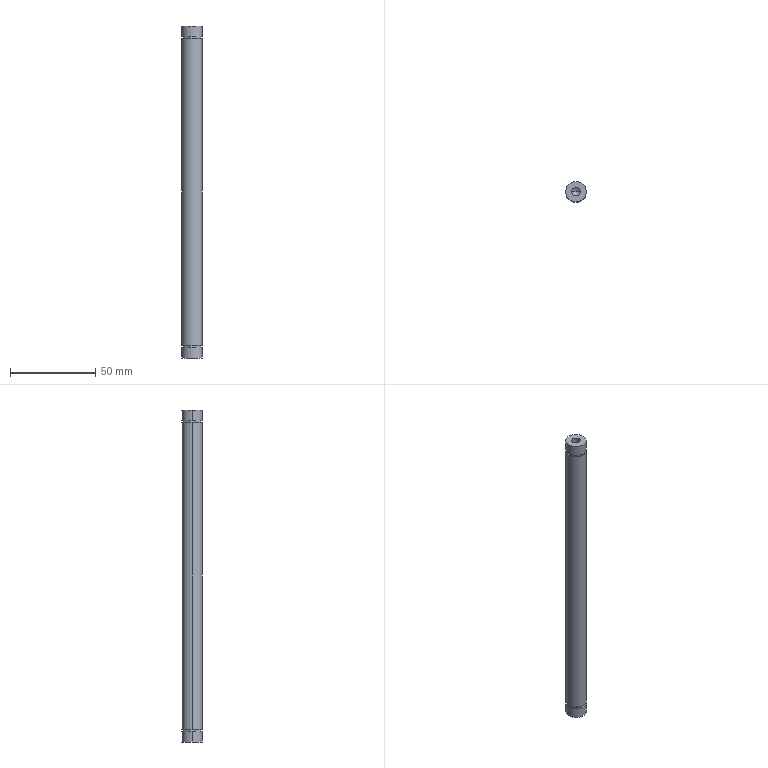Part | STEP file | MT-COMBO-119-S035 | 1 solid | 24 faces | box 12 x 12 x 195 mm | volume 21406 mm3 | cylinder 14 | plane 6 | cone 4 | commonest cylinder face diameters 12 x6 5 x4 11 x4
STEP:
#1=CARTESIAN_POINT('',(-6.,0.,6.4));
#2=VERTEX_POINT('',#1);
#3=CARTESIAN_POINT('',(6.,0.,6.4));
#4=VERTEX_POINT('',#3);
#5=CARTESIAN_POINT('',(0.,0.,6.4));
#6=DIRECTION('',(0.,0.,-1.));
#7=DIRECTION('',(-1.,0.,0.));
#8=AXIS2_PLACEMENT_3D('',#5,#6,#7);
#9=CIRCLE('',#8,6.);
#10=EDGE_CURVE('',#2,#4,#9,.T.);
#11=ORIENTED_EDGE('',*,*,#10,.T.);
#12=CARTESIAN_POINT('',(6.,0.,0.));
#13=VERTEX_POINT('',#12);
#14=CARTESIAN_POINT('',(6.,0.,195.));
#15=DIRECTION('',(0.,0.,-1.));
#16=VECTOR('',#15,1000.);
#17=LINE('',#14,#16);
#18=EDGE_CURVE('',#4,#13,#17,.T.);
#19=ORIENTED_EDGE('',*,*,#18,.T.);
#20=CARTESIAN_POINT('',(-6.,0.,0.));
#21=VERTEX_POINT('',#20);
#22=CARTESIAN_POINT('',(0.,0.,0.));
#23=DIRECTION('',(0.,0.,1.));
#24=DIRECTION('',(1.,0.,0.));
#25=AXIS2_PLACEMENT_3D('',#22,#23,#24);
#26=CIRCLE('',#25,6.);
#27=EDGE_CURVE('',#13,#21,#26,.T.);
#28=ORIENTED_EDGE('',*,*,#27,.T.);
#29=CARTESIAN_POINT('',(-6.,0.,195.));
#30=DIRECTION('',(0.,0.,-1.));
#31=VECTOR('',#30,1000.);
#32=LINE('',#29,#31);
#33=EDGE_CURVE('',#2,#21,#32,.T.);
#34=ORIENTED_EDGE('',*,*,#33,.F.);
#35=EDGE_LOOP('',(#11,#19,#28,#34));
#36=FACE_OUTER_BOUND('',#35,.T.);
#37=CARTESIAN_POINT('',(0.,0.,195.));
#38=DIRECTION('',(0.,0.,-1.));
#39=DIRECTION('',(-1.,0.,0.));
#40=AXIS2_PLACEMENT_3D('',#37,#38,#39);
#41=CYLINDRICAL_SURFACE('',#40,6.);
#42=ADVANCED_FACE('',(#36),#41,.T.);
#43=CARTESIAN_POINT('',(2.5,0.,15.));
#44=VERTEX_POINT('',#43);
#45=CARTESIAN_POINT('',(-2.5,0.,15.));
#46=VERTEX_POINT('',#45);
#47=CARTESIAN_POINT('',(0.,0.,15.));
#48=DIRECTION('',(0.,0.,-1.));
#49=DIRECTION('',(-1.,0.,0.));
#50=AXIS2_PLACEMENT_3D('',#47,#48,#49);
#51=CIRCLE('',#50,2.5);
#52=EDGE_CURVE('',#44,#46,#51,.T.);
#53=ORIENTED_EDGE('',*,*,#52,.F.);
#54=CARTESIAN_POINT('',(2.5,0.,0.));
#55=VERTEX_POINT('',#54);
#56=CARTESIAN_POINT('',(2.5,0.,0.));
#57=DIRECTION('',(0.,0.,-1.));
#58=VECTOR('',#57,1000.);
#59=LINE('',#56,#58);
#60=EDGE_CURVE('',#44,#55,#59,.T.);
#61=ORIENTED_EDGE('',*,*,#60,.T.);
#62=CARTESIAN_POINT('',(-2.5,0.,0.));
#63=VERTEX_POINT('',#62);
#64=CARTESIAN_POINT('',(0.,0.,0.));
#65=DIRECTION('',(0.,0.,-1.));
#66=DIRECTION('',(-1.,0.,0.));
#67=AXIS2_PLACEMENT_3D('',#64,#65,#66);
#68=CIRCLE('',#67,2.5);
#69=EDGE_CURVE('',#55,#63,#68,.T.);
#70=ORIENTED_EDGE('',*,*,#69,.T.);
#71=CARTESIAN_POINT('',(-2.5,0.,0.));
#72=DIRECTION('',(0.,0.,-1.));
#73=VECTOR('',#72,1000.);
#74=LINE('',#71,#73);
#75=EDGE_CURVE('',#46,#63,#74,.T.);
#76=ORIENTED_EDGE('',*,*,#75,.F.);
#77=EDGE_LOOP('',(#53,#61,#70,#76));
#78=FACE_OUTER_BOUND('',#77,.T.);
#79=CARTESIAN_POINT('',(0.,0.,0.));
#80=DIRECTION('',(0.,0.,-1.));
#81=DIRECTION('',(-1.,0.,0.));
#82=AXIS2_PLACEMENT_3D('',#79,#80,#81);
#83=CYLINDRICAL_SURFACE('',#82,2.5);
#84=ADVANCED_FACE('',(#78),#83,.F.);
#85=CARTESIAN_POINT('',(0.,0.,16.502));
#86=VERTEX_POINT('',#85);
#87=CARTESIAN_POINT('',(-2.5,0.,15.));
#88=DIRECTION('',(-0.8572,0.,-0.515));
#89=VECTOR('',#88,1000.);
#90=LINE('',#87,#89);
#91=EDGE_CURVE('',#86,#46,#90,.T.);
#92=ORIENTED_EDGE('',*,*,#91,.F.);
#93=CARTESIAN_POINT('',(2.5,0.,15.));
#94=DIRECTION('',(0.8572,0.,-0.515));
#95=VECTOR('',#94,1000.);
#96=LINE('',#93,#95);
#97=EDGE_CURVE('',#86,#44,#96,.T.);
#98=ORIENTED_EDGE('',*,*,#97,.T.);
#99=ORIENTED_EDGE('',*,*,#52,.T.);
#100=EDGE_LOOP('',(#92,#98,#99));
#101=FACE_OUTER_BOUND('',#100,.T.);
#102=CARTESIAN_POINT('',(0.,0.,15.));
#103=DIRECTION('',(0.,0.,-1.));
#104=DIRECTION('',(-1.,0.,0.));
#105=AXIS2_PLACEMENT_3D('',#102,#103,#104);
#106=CONICAL_SURFACE('',#105,2.5,1.03);
#107=ADVANCED_FACE('',(#101),#106,.F.);
#108=CARTESIAN_POINT('',(-5.5,0.,6.4));
#109=VERTEX_POINT('',#108);
#110=CARTESIAN_POINT('',(5.5,0.,6.4));
#111=VERTEX_POINT('',#110);
#112=CARTESIAN_POINT('',(0.,0.,6.4));
#113=DIRECTION('',(0.,0.,-1.));
#114=DIRECTION('',(-1.,0.,0.));
#115=AXIS2_PLACEMENT_3D('',#112,#113,#114);
#116=CIRCLE('',#115,5.5);
#117=EDGE_CURVE('',#109,#111,#116,.T.);
#118=ORIENTED_EDGE('',*,*,#117,.F.);
#119=CARTESIAN_POINT('',(-5.5,0.,7.5));
#120=VERTEX_POINT('',#119);
#121=CARTESIAN_POINT('',(-5.5,0.,6.4));
#122=DIRECTION('',(0.,0.,1.));
#123=VECTOR('',#122,1000.);
#124=LINE('',#121,#123);
#125=EDGE_CURVE('',#109,#120,#124,.T.);
#126=ORIENTED_EDGE('',*,*,#125,.T.);
#127=CARTESIAN_POINT('',(5.5,0.,7.5));
#128=VERTEX_POINT('',#127);
#129=CARTESIAN_POINT('',(0.,0.,7.5));
#130=DIRECTION('',(0.,0.,-1.));
#131=DIRECTION('',(-1.,0.,0.));
#132=AXIS2_PLACEMENT_3D('',#129,#130,#131);
#133=CIRCLE('',#132,5.5);
#134=EDGE_CURVE('',#120,#128,#133,.T.);
#135=ORIENTED_EDGE('',*,*,#134,.T.);
#136=CARTESIAN_POINT('',(5.5,0.,6.4));
#137=DIRECTION('',(0.,0.,1.));
#138=VECTOR('',#137,1000.);
#139=LINE('',#136,#138);
#140=EDGE_CURVE('',#111,#128,#139,.T.);
#141=ORIENTED_EDGE('',*,*,#140,.F.);
#142=EDGE_LOOP('',(#118,#126,#135,#141));
#143=FACE_OUTER_BOUND('',#142,.T.);
#144=CARTESIAN_POINT('',(0.,0.,6.4));
#145=DIRECTION('',(0.,0.,1.));
#146=DIRECTION('',(1.,0.,0.));
#147=AXIS2_PLACEMENT_3D('',#144,#145,#146);
#148=CYLINDRICAL_SURFACE('',#147,5.5);
#149=ADVANCED_FACE('',(#143),#148,.T.);
#150=CARTESIAN_POINT('',(5.5,0.,188.6));
#151=VERTEX_POINT('',#150);
#152=CARTESIAN_POINT('',(-5.5,0.,188.6));
#153=VERTEX_POINT('',#152);
#154=CARTESIAN_POINT('',(0.,0.,188.6));
#155=DIRECTION('',(0.,0.,1.));
#156=DIRECTION('',(1.,0.,0.));
#157=AXIS2_PLACEMENT_3D('',#154,#155,#156);
#158=CIRCLE('',#157,5.5);
#159=EDGE_CURVE('',#151,#153,#158,.T.);
#160=ORIENTED_EDGE('',*,*,#159,.F.);
#161=CARTESIAN_POINT('',(5.5,0.,187.5));
#162=VERTEX_POINT('',#161);
#163=CARTESIAN_POINT('',(5.5,0.,188.6));
#164=DIRECTION('',(0.,0.,-1.));
#165=VECTOR('',#164,1000.);
#166=LINE('',#163,#165);
#167=EDGE_CURVE('',#151,#162,#166,.T.);
#168=ORIENTED_EDGE('',*,*,#167,.T.);
#169=CARTESIAN_POINT('',(-5.5,0.,187.5));
#170=VERTEX_POINT('',#169);
#171=CARTESIAN_POINT('',(0.,0.,187.5));
#172=DIRECTION('',(0.,0.,1.));
#173=DIRECTION('',(1.,0.,0.));
#174=AXIS2_PLACEMENT_3D('',#171,#172,#173);
#175=CIRCLE('',#174,5.5);
#176=EDGE_CURVE('',#162,#170,#175,.T.);
#177=ORIENTED_EDGE('',*,*,#176,.T.);
#178=CARTESIAN_POINT('',(-5.5,0.,188.6));
#179=DIRECTION('',(0.,0.,-1.));
#180=VECTOR('',#179,1000.);
#181=LINE('',#178,#180);
#182=EDGE_CURVE('',#153,#170,#181,.T.);
#183=ORIENTED_EDGE('',*,*,#182,.F.);
#184=EDGE_LOOP('',(#160,#168,#177,#183));
#185=FACE_OUTER_BOUND('',#184,.T.);
#186=CARTESIAN_POINT('',(0.,0.,188.6));
#187=DIRECTION('',(0.,0.,-1.));
#188=DIRECTION('',(-1.,0.,0.));
#189=AXIS2_PLACEMENT_3D('',#186,#187,#188);
#190=CYLINDRICAL_SURFACE('',#189,5.5);
#191=ADVANCED_FACE('',(#185),#190,.T.);
#192=CARTESIAN_POINT('',(-2.5,0.,180.));
#193=VERTEX_POINT('',#192);
#194=CARTESIAN_POINT('',(2.5,0.,180.));
#195=VERTEX_POINT('',#194);
#196=CARTESIAN_POINT('',(0.,0.,180.));
#197=DIRECTION('',(0.,0.,1.));
#198=DIRECTION('',(1.,0.,0.));
#199=AXIS2_PLACEMENT_3D('',#196,#197,#198);
#200=CIRCLE('',#199,2.5);
#201=EDGE_CURVE('',#193,#195,#200,.T.);
#202=ORIENTED_EDGE('',*,*,#201,.F.);
#203=CARTESIAN_POINT('',(-2.5,0.,195.));
#204=VERTEX_POINT('',#203);
#205=CARTESIAN_POINT('',(-2.5,0.,195.));
#206=DIRECTION('',(0.,0.,1.));
#207=VECTOR('',#206,1000.);
#208=LINE('',#205,#207);
#209=EDGE_CURVE('',#193,#204,#208,.T.);
#210=ORIENTED_EDGE('',*,*,#209,.T.);
#211=CARTESIAN_POINT('',(2.5,0.,195.));
#212=VERTEX_POINT('',#211);
#213=CARTESIAN_POINT('',(0.,0.,195.));
#214=DIRECTION('',(0.,0.,1.));
#215=DIRECTION('',(1.,0.,0.));
#216=AXIS2_PLACEMENT_3D('',#213,#214,#215);
#217=CIRCLE('',#216,2.5);
#218=EDGE_CURVE('',#204,#212,#217,.T.);
#219=ORIENTED_EDGE('',*,*,#218,.T.);
#220=CARTESIAN_POINT('',(2.5,0.,195.));
#221=DIRECTION('',(0.,0.,1.));
#222=VECTOR('',#221,1000.);
#223=LINE('',#220,#222);
#224=EDGE_CURVE('',#195,#212,#223,.T.);
#225=ORIENTED_EDGE('',*,*,#224,.F.);
#226=EDGE_LOOP('',(#202,#210,#219,#225));
#227=FACE_OUTER_BOUND('',#226,.T.);
#228=CARTESIAN_POINT('',(0.,0.,195.));
#229=DIRECTION('',(0.,0.,1.));
#230=DIRECTION('',(1.,0.,0.));
#231=AXIS2_PLACEMENT_3D('',#228,#229,#230);
#232=CYLINDRICAL_SURFACE('',#231,2.5);
#233=ADVANCED_FACE('',(#227),#232,.F.);
#234=CARTESIAN_POINT('',(0.,0.,178.498));
#235=VERTEX_POINT('',#234);
#236=CARTESIAN_POINT('',(2.5,0.,180.));
#237=DIRECTION('',(0.8572,0.,0.515));
#238=VECTOR('',#237,1000.);
#239=LINE('',#236,#238);
#240=EDGE_CURVE('',#235,#195,#239,.T.);
#241=ORIENTED_EDGE('',*,*,#240,.F.);
#242=CARTESIAN_POINT('',(-2.5,0.,180.));
#243=DIRECTION('',(-0.8572,0.,0.515));
#244=VECTOR('',#243,1000.);
#245=LINE('',#242,#244);
#246=EDGE_CURVE('',#235,#193,#245,.T.);
#247=ORIENTED_EDGE('',*,*,#246,.T.);
#248=ORIENTED_EDGE('',*,*,#201,.T.);
#249=EDGE_LOOP('',(#241,#247,#248));
#250=FACE_OUTER_BOUND('',#249,.T.);
#251=CARTESIAN_POINT('',(0.,0.,180.));
#252=DIRECTION('',(0.,0.,1.));
#253=DIRECTION('',(1.,0.,0.));
#254=AXIS2_PLACEMENT_3D('',#251,#252,#253);
#255=CONICAL_SURFACE('',#254,2.5,1.03);
#256=ADVANCED_FACE('',(#250),#255,.F.);
#257=CARTESIAN_POINT('',(6.,0.,195.));
#258=VERTEX_POINT('',#257);
#259=CARTESIAN_POINT('',(-6.,0.,195.));
#260=VERTEX_POINT('',#259);
#261=CARTESIAN_POINT('',(0.,0.,195.));
#262=DIRECTION('',(0.,0.,1.));
#263=DIRECTION('',(1.,0.,0.));
#264=AXIS2_PLACEMENT_3D('',#261,#262,#263);
#265=CIRCLE('',#264,6.);
#266=EDGE_CURVE('',#258,#260,#265,.T.);
#267=ORIENTED_EDGE('',*,*,#266,.F.);
#268=CARTESIAN_POINT('',(6.,0.,188.6));
#269=VERTEX_POINT('',#268);
#270=CARTESIAN_POINT('',(6.,0.,195.));
#271=DIRECTION('',(0.,0.,-1.));
#272=VECTOR('',#271,1000.);
#273=LINE('',#270,#272);
#274=EDGE_CURVE('',#258,#269,#273,.T.);
#275=ORIENTED_EDGE('',*,*,#274,.T.);
#276=CARTESIAN_POINT('',(-6.,0.,188.6));
#277=VERTEX_POINT('',#276);
#278=CARTESIAN_POINT('',(0.,0.,188.6));
#279=DIRECTION('',(0.,0.,1.));
#280=DIRECTION('',(1.,0.,0.));
#281=AXIS2_PLACEMENT_3D('',#278,#279,#280);
#282=CIRCLE('',#281,6.);
#283=EDGE_CURVE('',#269,#277,#282,.T.);
#284=ORIENTED_EDGE('',*,*,#283,.T.);
#285=CARTESIAN_POINT('',(-6.,0.,195.));
#286=DIRECTION('',(0.,0.,-1.));
#287=VECTOR('',#286,1000.);
#288=LINE('',#285,#287);
#289=EDGE_CURVE('',#260,#277,#288,.T.);
#290=ORIENTED_EDGE('',*,*,#289,.F.);
#291=EDGE_LOOP('',(#267,#275,#284,#290));
#292=FACE_OUTER_BOUND('',#291,.T.);
#293=CARTESIAN_POINT('',(0.,0.,195.));
#294=DIRECTION('',(0.,0.,-1.));
#295=DIRECTION('',(-1.,0.,0.));
#296=AXIS2_PLACEMENT_3D('',#293,#294,#295);
#297=CYLINDRICAL_SURFACE('',#296,6.);
#298=ADVANCED_FACE('',(#292),#297,.T.);
#299=CARTESIAN_POINT('',(6.,0.,187.5));
#300=VERTEX_POINT('',#299);
#301=CARTESIAN_POINT('',(-6.,0.,187.5));
#302=VERTEX_POINT('',#301);
#303=CARTESIAN_POINT('',(0.,0.,187.5));
#304=DIRECTION('',(0.,0.,1.));
#305=DIRECTION('',(1.,0.,0.));
#306=AXIS2_PLACEMENT_3D('',#303,#304,#305);
#307=CIRCLE('',#306,6.);
#308=EDGE_CURVE('',#300,#302,#307,.T.);
#309=ORIENTED_EDGE('',*,*,#308,.F.);
#310=CARTESIAN_POINT('',(6.,0.,7.5));
#311=VERTEX_POINT('',#310);
#312=CARTESIAN_POINT('',(6.,0.,195.));
#313=DIRECTION('',(0.,0.,-1.));
#314=VECTOR('',#313,1000.);
#315=LINE('',#312,#314);
#316=EDGE_CURVE('',#300,#311,#315,.T.);
#317=ORIENTED_EDGE('',*,*,#316,.T.);
#318=CARTESIAN_POINT('',(-6.,0.,7.5));
#319=VERTEX_POINT('',#318);
#320=CARTESIAN_POINT('',(0.,0.,7.5));
#321=DIRECTION('',(0.,0.,-1.));
#322=DIRECTION('',(-1.,0.,0.));
#323=AXIS2_PLACEMENT_3D('',#320,#321,#322);
#324=CIRCLE('',#323,6.);
#325=EDGE_CURVE('',#319,#311,#324,.T.);
#326=ORIENTED_EDGE('',*,*,#325,.F.);
#327=CARTESIAN_POINT('',(-6.,0.,195.));
#328=DIRECTION('',(0.,0.,-1.));
#329=VECTOR('',#328,1000.);
#330=LINE('',#327,#329);
#331=EDGE_CURVE('',#302,#319,#330,.T.);
#332=ORIENTED_EDGE('',*,*,#331,.F.);
#333=EDGE_LOOP('',(#309,#317,#326,#332));
#334=FACE_OUTER_BOUND('',#333,.T.);
#335=CARTESIAN_POINT('',(0.,0.,195.));
#336=DIRECTION('',(0.,0.,-1.));
#337=DIRECTION('',(-1.,0.,0.));
#338=AXIS2_PLACEMENT_3D('',#335,#336,#337);
#339=CYLINDRICAL_SURFACE('',#338,6.);
#340=ADVANCED_FACE('',(#334),#339,.T.);
#341=ORIENTED_EDGE('',*,*,#316,.F.);
#342=CARTESIAN_POINT('',(0.,0.,187.5));
#343=DIRECTION('',(0.,0.,1.));
#344=DIRECTION('',(1.,0.,0.));
#345=AXIS2_PLACEMENT_3D('',#342,#343,#344);
#346=CIRCLE('',#345,6.);
#347=EDGE_CURVE('',#302,#300,#346,.T.);
#348=ORIENTED_EDGE('',*,*,#347,.F.);
#349=ORIENTED_EDGE('',*,*,#331,.T.);
#350=CARTESIAN_POINT('',(0.,0.,7.5));
#351=DIRECTION('',(0.,0.,-1.));
#352=DIRECTION('',(-1.,0.,0.));
#353=AXIS2_PLACEMENT_3D('',#350,#351,#352);
#354=CIRCLE('',#353,6.);
#355=EDGE_CURVE('',#311,#319,#354,.T.);
#356=ORIENTED_EDGE('',*,*,#355,.F.);
#357=EDGE_LOOP('',(#341,#348,#349,#356));
#358=FACE_OUTER_BOUND('',#357,.T.);
#359=CARTESIAN_POINT('',(0.,0.,195.));
#360=DIRECTION('',(0.,0.,-1.));
#361=DIRECTION('',(-1.,0.,0.));
#362=AXIS2_PLACEMENT_3D('',#359,#360,#361);
#363=CYLINDRICAL_SURFACE('',#362,6.);
#364=ADVANCED_FACE('',(#358),#363,.T.);
#365=ORIENTED_EDGE('',*,*,#274,.F.);
#366=CARTESIAN_POINT('',(0.,0.,195.));
#367=DIRECTION('',(0.,0.,1.));
#368=DIRECTION('',(1.,0.,0.));
#369=AXIS2_PLACEMENT_3D('',#366,#367,#368);
#370=CIRCLE('',#369,6.);
#371=EDGE_CURVE('',#260,#258,#370,.T.);
#372=ORIENTED_EDGE('',*,*,#371,.F.);
#373=ORIENTED_EDGE('',*,*,#289,.T.);
#374=CARTESIAN_POINT('',(0.,0.,188.6));
#375=DIRECTION('',(0.,0.,1.));
#376=DIRECTION('',(1.,0.,0.));
#377=AXIS2_PLACEMENT_3D('',#374,#375,#376);
#378=CIRCLE('',#377,6.);
#379=EDGE_CURVE('',#277,#269,#378,.T.);
#380=ORIENTED_EDGE('',*,*,#379,.T.);
#381=EDGE_LOOP('',(#365,#372,#373,#380));
#382=FACE_OUTER_BOUND('',#381,.T.);
#383=CARTESIAN_POINT('',(0.,0.,195.));
#384=DIRECTION('',(0.,0.,-1.));
#385=DIRECTION('',(-1.,0.,0.));
#386=AXIS2_PLACEMENT_3D('',#383,#384,#385);
#387=CYLINDRICAL_SURFACE('',#386,6.);
#388=ADVANCED_FACE('',(#382),#387,.T.);
#389=CARTESIAN_POINT('',(0.,0.,195.));
#390=DIRECTION('',(0.,0.,1.));
#391=DIRECTION('',(1.,0.,0.));
#392=AXIS2_PLACEMENT_3D('',#389,#390,#391);
#393=CIRCLE('',#392,2.5);
#394=EDGE_CURVE('',#212,#204,#393,.T.);
#395=ORIENTED_EDGE('',*,*,#394,.F.);
#396=ORIENTED_EDGE('',*,*,#218,.F.);
#397=EDGE_LOOP('',(#395,#396));
#398=FACE_BOUND('',#397,.T.);
#399=ORIENTED_EDGE('',*,*,#371,.T.);
#400=ORIENTED_EDGE('',*,*,#266,.T.);
#401=EDGE_LOOP('',(#399,#400));
#402=FACE_OUTER_BOUND('',#401,.T.);
#403=CARTESIAN_POINT('',(0.,0.,195.));
#404=DIRECTION('',(0.,0.,1.));
#405=DIRECTION('',(1.,0.,0.));
#406=AXIS2_PLACEMENT_3D('',#403,#404,#405);
#407=PLANE('',#406);
#408=ADVANCED_FACE('',(#398,#402),#407,.T.);
#409=ORIENTED_EDGE('',*,*,#246,.F.);
#410=ORIENTED_EDGE('',*,*,#240,.T.);
#411=CARTESIAN_POINT('',(0.,0.,180.));
#412=DIRECTION('',(0.,0.,1.));
#413=DIRECTION('',(1.,0.,0.));
#414=AXIS2_PLACEMENT_3D('',#411,#412,#413);
#415=CIRCLE('',#414,2.5);
#416=EDGE_CURVE('',#195,#193,#415,.T.);
#417=ORIENTED_EDGE('',*,*,#416,.T.);
#418=EDGE_LOOP('',(#409,#410,#417));
#419=FACE_OUTER_BOUND('',#418,.T.);
#420=CARTESIAN_POINT('',(0.,0.,180.));
#421=DIRECTION('',(0.,0.,1.));
#422=DIRECTION('',(1.,0.,0.));
#423=AXIS2_PLACEMENT_3D('',#420,#421,#422);
#424=CONICAL_SURFACE('',#423,2.5,1.03);
#425=ADVANCED_FACE('',(#419),#424,.F.);
#426=ORIENTED_EDGE('',*,*,#209,.F.);
#427=ORIENTED_EDGE('',*,*,#416,.F.);
#428=ORIENTED_EDGE('',*,*,#224,.T.);
#429=ORIENTED_EDGE('',*,*,#394,.T.);
#430=EDGE_LOOP('',(#426,#427,#428,#429));
#431=FACE_OUTER_BOUND('',#430,.T.);
#432=CARTESIAN_POINT('',(0.,0.,195.));
#433=DIRECTION('',(0.,0.,1.));
#434=DIRECTION('',(1.,0.,0.));
#435=AXIS2_PLACEMENT_3D('',#432,#433,#434);
#436=CYLINDRICAL_SURFACE('',#435,2.5);
#437=ADVANCED_FACE('',(#431),#436,.F.);
#438=ORIENTED_EDGE('',*,*,#379,.F.);
#439=ORIENTED_EDGE('',*,*,#283,.F.);
#440=EDGE_LOOP('',(#438,#439));
#441=FACE_OUTER_BOUND('',#440,.T.);
#442=CARTESIAN_POINT('',(0.,0.,188.6));
#443=DIRECTION('',(0.,0.,1.));
#444=DIRECTION('',(1.,0.,0.));
#445=AXIS2_PLACEMENT_3D('',#442,#443,#444);
#446=CIRCLE('',#445,5.5);
#447=EDGE_CURVE('',#153,#151,#446,.T.);
#448=ORIENTED_EDGE('',*,*,#447,.T.);
#449=ORIENTED_EDGE('',*,*,#159,.T.);
#450=EDGE_LOOP('',(#448,#449));
#451=FACE_BOUND('',#450,.T.);
#452=CARTESIAN_POINT('',(0.,0.,188.6));
#453=DIRECTION('',(0.,0.,1.));
#454=DIRECTION('',(1.,0.,0.));
#455=AXIS2_PLACEMENT_3D('',#452,#453,#454);
#456=PLANE('',#455);
#457=ADVANCED_FACE('',(#441,#451),#456,.F.);
#458=ORIENTED_EDGE('',*,*,#347,.T.);
#459=ORIENTED_EDGE('',*,*,#308,.T.);
#460=EDGE_LOOP('',(#458,#459));
#461=FACE_OUTER_BOUND('',#460,.T.);
#462=CARTESIAN_POINT('',(0.,0.,187.5));
#463=DIRECTION('',(0.,0.,1.));
#464=DIRECTION('',(1.,0.,0.));
#465=AXIS2_PLACEMENT_3D('',#462,#463,#464);
#466=CIRCLE('',#465,5.5);
#467=EDGE_CURVE('',#170,#162,#466,.T.);
#468=ORIENTED_EDGE('',*,*,#467,.F.);
#469=ORIENTED_EDGE('',*,*,#176,.F.);
#470=EDGE_LOOP('',(#468,#469));
#471=FACE_BOUND('',#470,.T.);
#472=CARTESIAN_POINT('',(0.,0.,187.5));
#473=DIRECTION('',(0.,0.,1.));
#474=DIRECTION('',(1.,0.,0.));
#475=AXIS2_PLACEMENT_3D('',#472,#473,#474);
#476=PLANE('',#475);
#477=ADVANCED_FACE('',(#461,#471),#476,.T.);
#478=ORIENTED_EDGE('',*,*,#167,.F.);
#479=ORIENTED_EDGE('',*,*,#447,.F.);
#480=ORIENTED_EDGE('',*,*,#182,.T.);
#481=ORIENTED_EDGE('',*,*,#467,.T.);
#482=EDGE_LOOP('',(#478,#479,#480,#481));
#483=FACE_OUTER_BOUND('',#482,.T.);
#484=CARTESIAN_POINT('',(0.,0.,188.6));
#485=DIRECTION('',(0.,0.,-1.));
#486=DIRECTION('',(-1.,0.,0.));
#487=AXIS2_PLACEMENT_3D('',#484,#485,#486);
#488=CYLINDRICAL_SURFACE('',#487,5.5);
#489=ADVANCED_FACE('',(#483),#488,.T.);
#490=ORIENTED_EDGE('',*,*,#10,.F.);
#491=CARTESIAN_POINT('',(0.,0.,6.4));
#492=DIRECTION('',(0.,0.,-1.));
#493=DIRECTION('',(-1.,0.,0.));
#494=AXIS2_PLACEMENT_3D('',#491,#492,#493);
#495=CIRCLE('',#494,6.);
#496=EDGE_CURVE('',#4,#2,#495,.T.);
#497=ORIENTED_EDGE('',*,*,#496,.F.);
#498=EDGE_LOOP('',(#490,#497));
#499=FACE_OUTER_BOUND('',#498,.T.);
#500=CARTESIAN_POINT('',(0.,0.,6.4));
#501=DIRECTION('',(0.,0.,-1.));
#502=DIRECTION('',(-1.,0.,0.));
#503=AXIS2_PLACEMENT_3D('',#500,#501,#502);
#504=CIRCLE('',#503,5.5);
#505=EDGE_CURVE('',#111,#109,#504,.T.);
#506=ORIENTED_EDGE('',*,*,#505,.T.);
#507=ORIENTED_EDGE('',*,*,#117,.T.);
#508=EDGE_LOOP('',(#506,#507));
#509=FACE_BOUND('',#508,.T.);
#510=CARTESIAN_POINT('',(0.,0.,6.4));
#511=DIRECTION('',(0.,0.,-1.));
#512=DIRECTION('',(-1.,0.,0.));
#513=AXIS2_PLACEMENT_3D('',#510,#511,#512);
#514=PLANE('',#513);
#515=ADVANCED_FACE('',(#499,#509),#514,.F.);
#516=ORIENTED_EDGE('',*,*,#325,.T.);
#517=ORIENTED_EDGE('',*,*,#355,.T.);
#518=EDGE_LOOP('',(#516,#517));
#519=FACE_OUTER_BOUND('',#518,.T.);
#520=CARTESIAN_POINT('',(0.,0.,7.5));
#521=DIRECTION('',(0.,0.,-1.));
#522=DIRECTION('',(-1.,0.,0.));
#523=AXIS2_PLACEMENT_3D('',#520,#521,#522);
#524=CIRCLE('',#523,5.5);
#525=EDGE_CURVE('',#128,#120,#524,.T.);
#526=ORIENTED_EDGE('',*,*,#525,.F.);
#527=ORIENTED_EDGE('',*,*,#134,.F.);
#528=EDGE_LOOP('',(#526,#527));
#529=FACE_BOUND('',#528,.T.);
#530=CARTESIAN_POINT('',(0.,0.,7.5));
#531=DIRECTION('',(0.,0.,-1.));
#532=DIRECTION('',(-1.,0.,0.));
#533=AXIS2_PLACEMENT_3D('',#530,#531,#532);
#534=PLANE('',#533);
#535=ADVANCED_FACE('',(#519,#529),#534,.T.);
#536=ORIENTED_EDGE('',*,*,#125,.F.);
#537=ORIENTED_EDGE('',*,*,#505,.F.);
#538=ORIENTED_EDGE('',*,*,#140,.T.);
#539=ORIENTED_EDGE('',*,*,#525,.T.);
#540=EDGE_LOOP('',(#536,#537,#538,#539));
#541=FACE_OUTER_BOUND('',#540,.T.);
#542=CARTESIAN_POINT('',(0.,0.,6.4));
#543=DIRECTION('',(0.,0.,1.));
#544=DIRECTION('',(1.,0.,0.));
#545=AXIS2_PLACEMENT_3D('',#542,#543,#544);
#546=CYLINDRICAL_SURFACE('',#545,5.5);
#547=ADVANCED_FACE('',(#541),#546,.T.);
#548=ORIENTED_EDGE('',*,*,#97,.F.);
#549=ORIENTED_EDGE('',*,*,#91,.T.);
#550=CARTESIAN_POINT('',(0.,0.,15.));
#551=DIRECTION('',(0.,0.,-1.));
#552=DIRECTION('',(-1.,0.,0.));
#553=AXIS2_PLACEMENT_3D('',#550,#551,#552);
#554=CIRCLE('',#553,2.5);
#555=EDGE_CURVE('',#46,#44,#554,.T.);
#556=ORIENTED_EDGE('',*,*,#555,.T.);
#557=EDGE_LOOP('',(#548,#549,#556));
#558=FACE_OUTER_BOUND('',#557,.T.);
#559=CARTESIAN_POINT('',(0.,0.,15.));
#560=DIRECTION('',(0.,0.,-1.));
#561=DIRECTION('',(-1.,0.,0.));
#562=AXIS2_PLACEMENT_3D('',#559,#560,#561);
#563=CONICAL_SURFACE('',#562,2.5,1.03);
#564=ADVANCED_FACE('',(#558),#563,.F.);
#565=ORIENTED_EDGE('',*,*,#60,.F.);
#566=ORIENTED_EDGE('',*,*,#555,.F.);
#567=ORIENTED_EDGE('',*,*,#75,.T.);
#568=CARTESIAN_POINT('',(0.,0.,0.));
#569=DIRECTION('',(0.,0.,-1.));
#570=DIRECTION('',(-1.,0.,0.));
#571=AXIS2_PLACEMENT_3D('',#568,#569,#570);
#572=CIRCLE('',#571,2.5);
#573=EDGE_CURVE('',#63,#55,#572,.T.);
#574=ORIENTED_EDGE('',*,*,#573,.T.);
#575=EDGE_LOOP('',(#565,#566,#567,#574));
#576=FACE_OUTER_BOUND('',#575,.T.);
#577=CARTESIAN_POINT('',(0.,0.,0.));
#578=DIRECTION('',(0.,0.,-1.));
#579=DIRECTION('',(-1.,0.,0.));
#580=AXIS2_PLACEMENT_3D('',#577,#578,#579);
#581=CYLINDRICAL_SURFACE('',#580,2.5);
#582=ADVANCED_FACE('',(#576),#581,.F.);
#583=ORIENTED_EDGE('',*,*,#573,.F.);
#584=ORIENTED_EDGE('',*,*,#69,.F.);
#585=EDGE_LOOP('',(#583,#584));
#586=FACE_BOUND('',#585,.T.);
#587=CARTESIAN_POINT('',(0.,0.,0.));
#588=DIRECTION('',(0.,0.,1.));
#589=DIRECTION('',(1.,0.,0.));
#590=AXIS2_PLACEMENT_3D('',#587,#588,#589);
#591=CIRCLE('',#590,6.);
#592=EDGE_CURVE('',#21,#13,#591,.T.);
#593=ORIENTED_EDGE('',*,*,#592,.F.);
#594=ORIENTED_EDGE('',*,*,#27,.F.);
#595=EDGE_LOOP('',(#593,#594));
#596=FACE_OUTER_BOUND('',#595,.T.);
#597=CARTESIAN_POINT('',(0.,0.,0.));
#598=DIRECTION('',(0.,0.,1.));
#599=DIRECTION('',(1.,0.,0.));
#600=AXIS2_PLACEMENT_3D('',#597,#598,#599);
#601=PLANE('',#600);
#602=ADVANCED_FACE('',(#586,#596),#601,.F.);
#603=ORIENTED_EDGE('',*,*,#18,.F.);
#604=ORIENTED_EDGE('',*,*,#496,.T.);
#605=ORIENTED_EDGE('',*,*,#33,.T.);
#606=ORIENTED_EDGE('',*,*,#592,.T.);
#607=EDGE_LOOP('',(#603,#604,#605,#606));
#608=FACE_OUTER_BOUND('',#607,.T.);
#609=CARTESIAN_POINT('',(0.,0.,195.));
#610=DIRECTION('',(0.,0.,-1.));
#611=DIRECTION('',(-1.,0.,0.));
#612=AXIS2_PLACEMENT_3D('',#609,#610,#611);
#613=CYLINDRICAL_SURFACE('',#612,6.);
#614=ADVANCED_FACE('',(#608),#613,.T.);
#615=CLOSED_SHELL('',(#42,#84,#107,#149,#191,#233,#256,#298,#340,#364,#388,#408,#425,#437,#457,#477,#489,#515,#535,#547,#564,#582,#602,#614));
#616=MANIFOLD_SOLID_BREP('',#615);
#617=CARTESIAN_POINT('',(0.,0.,0.));
#618=DIRECTION('',(0.,0.,1.));
#619=DIRECTION('',(1.,0.,0.));
#620=AXIS2_PLACEMENT_3D('',#617,#618,#619);
#621=(LENGTH_UNIT()NAMED_UNIT(*)SI_UNIT(.MILLI.,.METRE.));
#622=UNCERTAINTY_MEASURE_WITH_UNIT(LENGTH_MEASURE(0.00001),#621,'','');
#623=(NAMED_UNIT(*)PLANE_ANGLE_UNIT()SI_UNIT($,.RADIAN.));
#624=(NAMED_UNIT(*)SI_UNIT($,.STERADIAN.)SOLID_ANGLE_UNIT());
#625=(GEOMETRIC_REPRESENTATION_CONTEXT(3)GLOBAL_UNCERTAINTY_ASSIGNED_CONTEXT((#622))GLOBAL_UNIT_ASSIGNED_CONTEXT((#621,#623,#624))REPRESENTATION_CONTEXT('',''));
#626=ADVANCED_BREP_SHAPE_REPRESENTATION('',(#616,#620),#625);